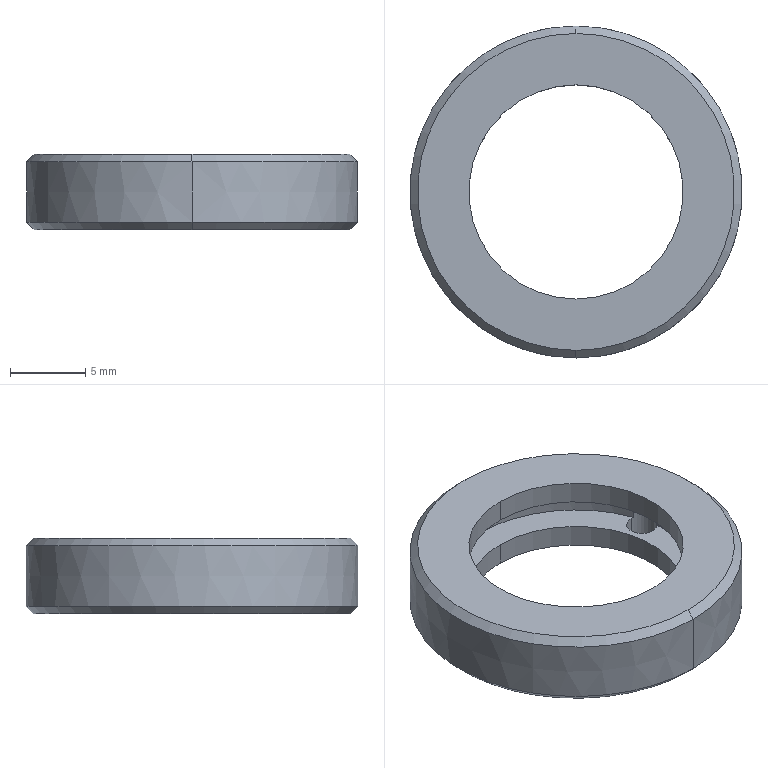Part | SolidWorks | features BaseBody 1 | 1 solid | 22 faces | box 22 x 22 x 5 mm | volume 889.388 mm3 | cylinder 10 | cone 6 | plane 6 | commonest cylinder face diameters 2 x4 14.2 x4 18 x2
STEP:
#1=CARTESIAN_POINT('',(558.371,-163.427,249.045));
#2=VERTEX_POINT('',#1);
#3=CARTESIAN_POINT('',(558.371,-184.426,249.045));
#4=VERTEX_POINT('',#3);
#5=CARTESIAN_POINT('',(558.371,-173.927,249.045));
#6=DIRECTION('',(0.000000003,0.000000023,-1.));
#7=DIRECTION('',(0.,1.,0.000000023));
#8=AXIS2_PLACEMENT_3D('',#5,#6,#7);
#9=CIRCLE('',#8,10.5);
#10=EDGE_CURVE('',#2,#4,#9,.T.);
#11=ORIENTED_EDGE('',*,*,#10,.T.);
#12=CARTESIAN_POINT('',(558.371,-184.926,248.544));
#13=VERTEX_POINT('',#12);
#14=CARTESIAN_POINT('',(558.371,-184.926,248.544));
#15=DIRECTION('',(0.000000002,-0.707,-0.7072));
#16=VECTOR('',#15,1000.);
#17=LINE('',#14,#16);
#18=EDGE_CURVE('',#4,#13,#17,.T.);
#19=ORIENTED_EDGE('',*,*,#18,.T.);
#20=CARTESIAN_POINT('',(558.371,-162.927,248.544));
#21=VERTEX_POINT('',#20);
#22=CARTESIAN_POINT('',(558.371,-173.927,248.544));
#23=DIRECTION('',(-0.000000003,-0.000000023,1.));
#24=DIRECTION('',(-0.9579,-0.287,-0.000000009));
#25=AXIS2_PLACEMENT_3D('',#22,#23,#24);
#26=CIRCLE('',#25,11.);
#27=EDGE_CURVE('',#13,#21,#26,.T.);
#28=ORIENTED_EDGE('',*,*,#27,.T.);
#29=CARTESIAN_POINT('',(558.371,-162.927,248.544));
#30=DIRECTION('',(0.000000002,0.707,-0.7072));
#31=VECTOR('',#30,1000.);
#32=LINE('',#29,#31);
#33=EDGE_CURVE('',#2,#21,#32,.T.);
#34=ORIENTED_EDGE('',*,*,#33,.F.);
#35=EDGE_LOOP('',(#11,#19,#28,#34));
#36=FACE_OUTER_BOUND('',#35,.T.);
#37=CARTESIAN_POINT('',(558.371,-173.927,248.544));
#38=DIRECTION('',(0.000000003,0.000000023,-1.));
#39=DIRECTION('',(0.,1.,0.000000023));
#40=AXIS2_PLACEMENT_3D('',#37,#38,#39);
#41=CONICAL_SURFACE('',#40,11.,0.7853);
#42=ADVANCED_FACE('',(#36),#41,.T.);
#43=CARTESIAN_POINT('',(558.371,-166.827,247.545));
#44=VERTEX_POINT('',#43);
#45=CARTESIAN_POINT('',(558.371,-181.027,247.545));
#46=VERTEX_POINT('',#45);
#47=CARTESIAN_POINT('',(558.371,-173.927,247.545));
#48=DIRECTION('',(-0.000000003,-0.000000023,1.));
#49=DIRECTION('',(0.,-1.,-0.000000023));
#50=AXIS2_PLACEMENT_3D('',#47,#48,#49);
#51=CIRCLE('',#50,7.1);
#52=EDGE_CURVE('',#44,#46,#51,.T.);
#53=ORIENTED_EDGE('',*,*,#52,.F.);
#54=CARTESIAN_POINT('',(558.371,-166.827,249.045));
#55=VERTEX_POINT('',#54);
#56=CARTESIAN_POINT('',(558.371,-166.827,244.045));
#57=DIRECTION('',(-0.000000003,-0.000000023,1.));
#58=VECTOR('',#57,1000.);
#59=LINE('',#56,#58);
#60=EDGE_CURVE('',#44,#55,#59,.T.);
#61=ORIENTED_EDGE('',*,*,#60,.T.);
#62=CARTESIAN_POINT('',(558.371,-181.027,249.045));
#63=VERTEX_POINT('',#62);
#64=CARTESIAN_POINT('',(558.371,-173.927,249.045));
#65=DIRECTION('',(-0.000000003,-0.000000023,1.));
#66=DIRECTION('',(0.,-1.,-0.000000023));
#67=AXIS2_PLACEMENT_3D('',#64,#65,#66);
#68=CIRCLE('',#67,7.1);
#69=EDGE_CURVE('',#55,#63,#68,.T.);
#70=ORIENTED_EDGE('',*,*,#69,.T.);
#71=CARTESIAN_POINT('',(558.371,-181.027,244.045));
#72=DIRECTION('',(-0.000000003,-0.000000023,1.));
#73=VECTOR('',#72,1000.);
#74=LINE('',#71,#73);
#75=EDGE_CURVE('',#46,#63,#74,.T.);
#76=ORIENTED_EDGE('',*,*,#75,.F.);
#77=EDGE_LOOP('',(#53,#61,#70,#76));
#78=FACE_OUTER_BOUND('',#77,.T.);
#79=CARTESIAN_POINT('',(558.371,-173.927,244.045));
#80=DIRECTION('',(-0.000000003,-0.000000023,1.));
#81=DIRECTION('',(0.,-1.,-0.000000023));
#82=AXIS2_PLACEMENT_3D('',#79,#80,#81);
#83=CYLINDRICAL_SURFACE('',#82,7.1);
#84=ADVANCED_FACE('',(#78),#83,.F.);
#85=CARTESIAN_POINT('',(558.371,-184.926,244.545));
#86=VERTEX_POINT('',#85);
#87=CARTESIAN_POINT('',(558.371,-162.927,244.545));
#88=VERTEX_POINT('',#87);
#89=CARTESIAN_POINT('',(558.371,-173.927,244.545));
#90=DIRECTION('',(-0.000000003,-0.000000023,1.));
#91=DIRECTION('',(-0.9579,-0.287,-0.000000009));
#92=AXIS2_PLACEMENT_3D('',#89,#90,#91);
#93=CIRCLE('',#92,10.999);
#94=EDGE_CURVE('',#86,#88,#93,.T.);
#95=ORIENTED_EDGE('',*,*,#94,.T.);
#96=CARTESIAN_POINT('',(558.371,-162.927,248.544));
#97=DIRECTION('',(-0.000000003,0.0001745,1.));
#98=VECTOR('',#97,1000.);
#99=LINE('',#96,#98);
#100=EDGE_CURVE('',#88,#21,#99,.T.);
#101=ORIENTED_EDGE('',*,*,#100,.T.);
#102=ORIENTED_EDGE('',*,*,#27,.F.);
#103=CARTESIAN_POINT('',(558.371,-184.926,248.544));
#104=DIRECTION('',(-0.000000003,-0.0001746,1.));
#105=VECTOR('',#104,1000.);
#106=LINE('',#103,#105);
#107=EDGE_CURVE('',#86,#13,#106,.T.);
#108=ORIENTED_EDGE('',*,*,#107,.F.);
#109=EDGE_LOOP('',(#95,#101,#102,#108));
#110=FACE_OUTER_BOUND('',#109,.T.);
#111=CARTESIAN_POINT('',(558.371,-173.927,248.544));
#112=DIRECTION('',(-0.000000003,-0.000000023,1.));
#113=DIRECTION('',(0.,-1.,-0.000000023));
#114=AXIS2_PLACEMENT_3D('',#111,#112,#113);
#115=CONICAL_SURFACE('',#114,11.,0.0001745);
#116=ADVANCED_FACE('',(#110),#115,.T.);
#117=CARTESIAN_POINT('',(558.371,-184.426,244.045));
#118=VERTEX_POINT('',#117);
#119=CARTESIAN_POINT('',(558.371,-163.427,244.045));
#120=VERTEX_POINT('',#119);
#121=CARTESIAN_POINT('',(558.371,-173.927,244.045));
#122=DIRECTION('',(-0.000000003,-0.000000023,1.));
#123=DIRECTION('',(0.,-1.,-0.000000023));
#124=AXIS2_PLACEMENT_3D('',#121,#122,#123);
#125=CIRCLE('',#124,10.499);
#126=EDGE_CURVE('',#118,#120,#125,.T.);
#127=ORIENTED_EDGE('',*,*,#126,.T.);
#128=CARTESIAN_POINT('',(558.371,-162.927,244.545));
#129=DIRECTION('',(-0.000000002,0.7072,0.707));
#130=VECTOR('',#129,1000.);
#131=LINE('',#128,#130);
#132=EDGE_CURVE('',#120,#88,#131,.T.);
#133=ORIENTED_EDGE('',*,*,#132,.T.);
#134=ORIENTED_EDGE('',*,*,#94,.F.);
#135=CARTESIAN_POINT('',(558.371,-184.926,244.545));
#136=DIRECTION('',(-0.000000002,-0.7072,0.707));
#137=VECTOR('',#136,1000.);
#138=LINE('',#135,#137);
#139=EDGE_CURVE('',#118,#86,#138,.T.);
#140=ORIENTED_EDGE('',*,*,#139,.F.);
#141=EDGE_LOOP('',(#127,#133,#134,#140));
#142=FACE_OUTER_BOUND('',#141,.T.);
#143=CARTESIAN_POINT('',(558.371,-173.927,244.545));
#144=DIRECTION('',(-0.000000003,-0.000000023,1.));
#145=DIRECTION('',(0.,-1.,-0.000000023));
#146=AXIS2_PLACEMENT_3D('',#143,#144,#145);
#147=CONICAL_SURFACE('',#146,10.999,0.7855);
#148=ADVANCED_FACE('',(#142),#147,.T.);
#149=CARTESIAN_POINT('',(558.371,-164.927,247.545));
#150=VERTEX_POINT('',#149);
#151=CARTESIAN_POINT('',(558.371,-182.927,247.545));
#152=VERTEX_POINT('',#151);
#153=CARTESIAN_POINT('',(558.371,-173.927,247.545));
#154=DIRECTION('',(-0.000000003,-0.000000023,1.));
#155=DIRECTION('',(0.,1.,0.000000023));
#156=AXIS2_PLACEMENT_3D('',#153,#154,#155);
#157=CIRCLE('',#156,9.);
#158=EDGE_CURVE('',#150,#152,#157,.T.);
#159=ORIENTED_EDGE('',*,*,#158,.T.);
#160=CARTESIAN_POINT('',(558.371,-182.927,245.545));
#161=VERTEX_POINT('',#160);
#162=CARTESIAN_POINT('',(558.371,-182.927,245.545));
#163=DIRECTION('',(0.000000003,0.000000023,-1.));
#164=VECTOR('',#163,1000.);
#165=LINE('',#162,#164);
#166=EDGE_CURVE('',#152,#161,#165,.T.);
#167=ORIENTED_EDGE('',*,*,#166,.T.);
#168=CARTESIAN_POINT('',(549.904,-176.978,245.545));
#169=VERTEX_POINT('',#168);
#170=CARTESIAN_POINT('',(558.371,-173.927,245.545));
#171=DIRECTION('',(-0.000000003,-0.000000023,1.));
#172=DIRECTION('',(0.,1.,0.000000023));
#173=AXIS2_PLACEMENT_3D('',#170,#171,#172);
#174=CIRCLE('',#173,9.);
#175=EDGE_CURVE('',#169,#161,#174,.T.);
#176=ORIENTED_EDGE('',*,*,#175,.F.);
#177=CARTESIAN_POINT('',(549.904,-176.978,246.045));
#178=VERTEX_POINT('',#177);
#179=CARTESIAN_POINT('',(549.904,-176.978,244.045));
#180=DIRECTION('',(-0.000000003,-0.000000023,1.));
#181=VECTOR('',#180,1000.);
#182=LINE('',#179,#181);
#183=EDGE_CURVE('',#169,#178,#182,.T.);
#184=ORIENTED_EDGE('',*,*,#183,.T.);
#185=CARTESIAN_POINT('',(549.469,-175.252,246.045));
#186=VERTEX_POINT('',#185);
#187=CARTESIAN_POINT('',(558.371,-173.927,246.045));
#188=DIRECTION('',(-0.000000003,-0.000000023,1.));
#189=DIRECTION('',(0.,1.,0.000000023));
#190=AXIS2_PLACEMENT_3D('',#187,#188,#189);
#191=CIRCLE('',#190,9.);
#192=EDGE_CURVE('',#186,#178,#191,.T.);
#193=ORIENTED_EDGE('',*,*,#192,.F.);
#194=CARTESIAN_POINT('',(549.469,-175.252,245.545));
#195=VERTEX_POINT('',#194);
#196=CARTESIAN_POINT('',(549.469,-175.252,244.045));
#197=DIRECTION('',(0.000000003,0.000000023,-1.));
#198=VECTOR('',#197,1000.);
#199=LINE('',#196,#198);
#200=EDGE_CURVE('',#186,#195,#199,.T.);
#201=ORIENTED_EDGE('',*,*,#200,.T.);
#202=CARTESIAN_POINT('',(558.371,-164.927,245.545));
#203=VERTEX_POINT('',#202);
#204=CARTESIAN_POINT('',(558.371,-173.927,245.545));
#205=DIRECTION('',(-0.000000003,-0.000000023,1.));
#206=DIRECTION('',(0.,1.,0.000000023));
#207=AXIS2_PLACEMENT_3D('',#204,#205,#206);
#208=CIRCLE('',#207,9.);
#209=EDGE_CURVE('',#203,#195,#208,.T.);
#210=ORIENTED_EDGE('',*,*,#209,.F.);
#211=CARTESIAN_POINT('',(558.371,-164.927,245.545));
#212=DIRECTION('',(0.000000003,0.000000023,-1.));
#213=VECTOR('',#212,1000.);
#214=LINE('',#211,#213);
#215=EDGE_CURVE('',#150,#203,#214,.T.);
#216=ORIENTED_EDGE('',*,*,#215,.F.);
#217=EDGE_LOOP('',(#159,#167,#176,#184,#193,#201,#210,#216));
#218=FACE_OUTER_BOUND('',#217,.T.);
#219=CARTESIAN_POINT('',(558.371,-173.927,245.545));
#220=DIRECTION('',(0.000000003,0.000000023,-1.));
#221=DIRECTION('',(0.,1.,0.000000023));
#222=AXIS2_PLACEMENT_3D('',#219,#220,#221);
#223=CYLINDRICAL_SURFACE('',#222,9.);
#224=ADVANCED_FACE('',(#218),#223,.F.);
#225=CARTESIAN_POINT('',(558.371,-166.827,244.045));
#226=VERTEX_POINT('',#225);
#227=CARTESIAN_POINT('',(558.371,-181.027,244.045));
#228=VERTEX_POINT('',#227);
#229=CARTESIAN_POINT('',(558.371,-173.927,244.045));
#230=DIRECTION('',(-0.000000003,-0.000000023,1.));
#231=DIRECTION('',(0.,-1.,-0.000000023));
#232=AXIS2_PLACEMENT_3D('',#229,#230,#231);
#233=CIRCLE('',#232,7.1);
#234=EDGE_CURVE('',#226,#228,#233,.T.);
#235=ORIENTED_EDGE('',*,*,#234,.F.);
#236=CARTESIAN_POINT('',(558.371,-166.827,245.545));
#237=VERTEX_POINT('',#236);
#238=CARTESIAN_POINT('',(558.371,-166.827,244.045));
#239=DIRECTION('',(-0.000000003,-0.000000023,1.));
#240=VECTOR('',#239,1000.);
#241=LINE('',#238,#240);
#242=EDGE_CURVE('',#226,#237,#241,.T.);
#243=ORIENTED_EDGE('',*,*,#242,.T.);
#244=CARTESIAN_POINT('',(558.371,-181.027,245.545));
#245=VERTEX_POINT('',#244);
#246=CARTESIAN_POINT('',(558.371,-173.927,245.545));
#247=DIRECTION('',(0.000000003,0.000000023,-1.));
#248=DIRECTION('',(0.,-1.,-0.000000023));
#249=AXIS2_PLACEMENT_3D('',#246,#247,#248);
#250=CIRCLE('',#249,7.1);
#251=EDGE_CURVE('',#245,#237,#250,.T.);
#252=ORIENTED_EDGE('',*,*,#251,.F.);
#253=CARTESIAN_POINT('',(558.371,-181.027,244.045));
#254=DIRECTION('',(-0.000000003,-0.000000023,1.));
#255=VECTOR('',#254,1000.);
#256=LINE('',#253,#255);
#257=EDGE_CURVE('',#228,#245,#256,.T.);
#258=ORIENTED_EDGE('',*,*,#257,.F.);
#259=EDGE_LOOP('',(#235,#243,#252,#258));
#260=FACE_OUTER_BOUND('',#259,.T.);
#261=CARTESIAN_POINT('',(558.371,-173.927,244.045));
#262=DIRECTION('',(-0.000000003,-0.000000023,1.));
#263=DIRECTION('',(0.,-1.,-0.000000023));
#264=AXIS2_PLACEMENT_3D('',#261,#262,#263);
#265=CYLINDRICAL_SURFACE('',#264,7.1);
#266=ADVANCED_FACE('',(#260),#265,.F.);
#267=CARTESIAN_POINT('',(566.613,-172.849,245.545));
#268=VERTEX_POINT('',#267);
#269=CARTESIAN_POINT('',(566.613,-170.849,245.545));
#270=VERTEX_POINT('',#269);
#271=CARTESIAN_POINT('',(566.613,-171.849,245.545));
#272=DIRECTION('',(0.000000003,0.000000023,-1.));
#273=DIRECTION('',(0.,1.,0.000000023));
#274=AXIS2_PLACEMENT_3D('',#271,#272,#273);
#275=CIRCLE('',#274,1.);
#276=EDGE_CURVE('',#268,#270,#275,.T.);
#277=ORIENTED_EDGE('',*,*,#276,.F.);
#278=CARTESIAN_POINT('',(566.613,-172.849,244.045));
#279=VERTEX_POINT('',#278);
#280=CARTESIAN_POINT('',(566.613,-172.849,244.045));
#281=DIRECTION('',(0.000000003,0.000000023,-1.));
#282=VECTOR('',#281,1000.);
#283=LINE('',#280,#282);
#284=EDGE_CURVE('',#268,#279,#283,.T.);
#285=ORIENTED_EDGE('',*,*,#284,.T.);
#286=CARTESIAN_POINT('',(566.613,-170.849,244.045));
#287=VERTEX_POINT('',#286);
#288=CARTESIAN_POINT('',(566.613,-171.849,244.045));
#289=DIRECTION('',(-0.000000003,-0.000000023,1.));
#290=DIRECTION('',(0.,1.,0.000000023));
#291=AXIS2_PLACEMENT_3D('',#288,#289,#290);
#292=CIRCLE('',#291,1.);
#293=EDGE_CURVE('',#287,#279,#292,.T.);
#294=ORIENTED_EDGE('',*,*,#293,.F.);
#295=CARTESIAN_POINT('',(566.613,-170.849,244.045));
#296=DIRECTION('',(0.000000003,0.000000023,-1.));
#297=VECTOR('',#296,1000.);
#298=LINE('',#295,#297);
#299=EDGE_CURVE('',#270,#287,#298,.T.);
#300=ORIENTED_EDGE('',*,*,#299,.F.);
#301=EDGE_LOOP('',(#277,#285,#294,#300));
#302=FACE_OUTER_BOUND('',#301,.T.);
#303=CARTESIAN_POINT('',(566.613,-171.849,244.045));
#304=DIRECTION('',(0.000000003,0.000000023,-1.));
#305=DIRECTION('',(0.,1.,0.000000023));
#306=AXIS2_PLACEMENT_3D('',#303,#304,#305);
#307=CYLINDRICAL_SURFACE('',#306,1.);
#308=ADVANCED_FACE('',(#302),#307,.F.);
#309=CARTESIAN_POINT('',(550.129,-177.004,245.545));
#310=VERTEX_POINT('',#309);
#311=CARTESIAN_POINT('',(550.129,-176.004,245.545));
#312=DIRECTION('',(0.000000003,0.000000023,-1.));
#313=DIRECTION('',(0.,1.,0.000000023));
#314=AXIS2_PLACEMENT_3D('',#311,#312,#313);
#315=CIRCLE('',#314,1.);
#316=EDGE_CURVE('',#310,#169,#315,.T.);
#317=ORIENTED_EDGE('',*,*,#316,.F.);
#318=CARTESIAN_POINT('',(550.129,-177.004,244.045));
#319=VERTEX_POINT('',#318);
#320=CARTESIAN_POINT('',(550.129,-177.004,244.045));
#321=DIRECTION('',(0.000000003,0.000000023,-1.));
#322=VECTOR('',#321,1000.);
#323=LINE('',#320,#322);
#324=EDGE_CURVE('',#310,#319,#323,.T.);
#325=ORIENTED_EDGE('',*,*,#324,.T.);
#326=CARTESIAN_POINT('',(550.129,-175.004,244.045));
#327=VERTEX_POINT('',#326);
#328=CARTESIAN_POINT('',(550.129,-176.004,244.045));
#329=DIRECTION('',(-0.000000003,-0.000000023,1.));
#330=DIRECTION('',(0.,1.,0.000000023));
#331=AXIS2_PLACEMENT_3D('',#328,#329,#330);
#332=CIRCLE('',#331,1.);
#333=EDGE_CURVE('',#327,#319,#332,.T.);
#334=ORIENTED_EDGE('',*,*,#333,.F.);
#335=CARTESIAN_POINT('',(550.129,-175.004,245.545));
#336=VERTEX_POINT('',#335);
#337=CARTESIAN_POINT('',(550.129,-175.004,244.045));
#338=DIRECTION('',(0.000000003,0.000000023,-1.));
#339=VECTOR('',#338,1000.);
#340=LINE('',#337,#339);
#341=EDGE_CURVE('',#336,#327,#340,.T.);
#342=ORIENTED_EDGE('',*,*,#341,.F.);
#343=CARTESIAN_POINT('',(550.129,-176.004,245.545));
#344=DIRECTION('',(0.000000003,0.000000023,-1.));
#345=DIRECTION('',(0.,1.,0.000000023));
#346=AXIS2_PLACEMENT_3D('',#343,#344,#345);
#347=CIRCLE('',#346,1.);
#348=EDGE_CURVE('',#195,#336,#347,.T.);
#349=ORIENTED_EDGE('',*,*,#348,.F.);
#350=ORIENTED_EDGE('',*,*,#200,.F.);
#351=CARTESIAN_POINT('',(550.129,-176.004,246.045));
#352=DIRECTION('',(-0.000000003,-0.000000023,1.));
#353=DIRECTION('',(0.,1.,0.000000023));
#354=AXIS2_PLACEMENT_3D('',#351,#352,#353);
#355=CIRCLE('',#354,1.);
#356=EDGE_CURVE('',#186,#178,#355,.T.);
#357=ORIENTED_EDGE('',*,*,#356,.T.);
#358=ORIENTED_EDGE('',*,*,#183,.F.);
#359=EDGE_LOOP('',(#317,#325,#334,#342,#349,#350,#357,#358));
#360=FACE_OUTER_BOUND('',#359,.T.);
#361=CARTESIAN_POINT('',(550.129,-176.004,244.045));
#362=DIRECTION('',(0.000000003,0.000000023,-1.));
#363=DIRECTION('',(0.,1.,0.000000023));
#364=AXIS2_PLACEMENT_3D('',#361,#362,#363);
#365=CYLINDRICAL_SURFACE('',#364,1.);
#366=ADVANCED_FACE('',(#360),#365,.F.);
#367=ORIENTED_EDGE('',*,*,#10,.F.);
#368=CARTESIAN_POINT('',(558.371,-173.927,249.045));
#369=DIRECTION('',(0.000000003,0.000000023,-1.));
#370=DIRECTION('',(0.,1.,0.000000023));
#371=AXIS2_PLACEMENT_3D('',#368,#369,#370);
#372=CIRCLE('',#371,10.5);
#373=EDGE_CURVE('',#4,#2,#372,.T.);
#374=ORIENTED_EDGE('',*,*,#373,.F.);
#375=EDGE_LOOP('',(#367,#374));
#376=FACE_OUTER_BOUND('',#375,.T.);
#377=CARTESIAN_POINT('',(558.371,-173.927,249.045));
#378=DIRECTION('',(-0.000000003,-0.000000023,1.));
#379=DIRECTION('',(0.,-1.,-0.000000023));
#380=AXIS2_PLACEMENT_3D('',#377,#378,#379);
#381=CIRCLE('',#380,7.1);
#382=EDGE_CURVE('',#63,#55,#381,.T.);
#383=ORIENTED_EDGE('',*,*,#382,.F.);
#384=ORIENTED_EDGE('',*,*,#69,.F.);
#385=EDGE_LOOP('',(#383,#384));
#386=FACE_BOUND('',#385,.T.);
#387=CARTESIAN_POINT('',(558.371,-173.927,249.045));
#388=DIRECTION('',(0.000000003,0.000000023,-1.));
#389=DIRECTION('',(0.,1.,0.000000023));
#390=AXIS2_PLACEMENT_3D('',#387,#388,#389);
#391=PLANE('',#390);
#392=ADVANCED_FACE('',(#376,#386),#391,.F.);
#393=ORIENTED_EDGE('',*,*,#18,.F.);
#394=ORIENTED_EDGE('',*,*,#373,.T.);
#395=ORIENTED_EDGE('',*,*,#33,.T.);
#396=CARTESIAN_POINT('',(558.371,-173.927,248.544));
#397=DIRECTION('',(-0.000000003,-0.000000023,1.));
#398=DIRECTION('',(-0.9579,-0.287,-0.000000009));
#399=AXIS2_PLACEMENT_3D('',#396,#397,#398);
#400=CIRCLE('',#399,11.);
#401=EDGE_CURVE('',#21,#13,#400,.T.);
#402=ORIENTED_EDGE('',*,*,#401,.T.);
#403=EDGE_LOOP('',(#393,#394,#395,#402));
#404=FACE_OUTER_BOUND('',#403,.T.);
#405=CARTESIAN_POINT('',(558.371,-173.927,248.544));
#406=DIRECTION('',(0.000000003,0.000000023,-1.));
#407=DIRECTION('',(0.,1.,0.000000023));
#408=AXIS2_PLACEMENT_3D('',#405,#406,#407);
#409=CONICAL_SURFACE('',#408,11.,0.7853);
#410=ADVANCED_FACE('',(#404),#409,.T.);
#411=ORIENTED_EDGE('',*,*,#60,.F.);
#412=CARTESIAN_POINT('',(558.371,-173.927,247.545));
#413=DIRECTION('',(-0.000000003,-0.000000023,1.));
#414=DIRECTION('',(0.,-1.,-0.000000023));
#415=AXIS2_PLACEMENT_3D('',#412,#413,#414);
#416=CIRCLE('',#415,7.1);
#417=EDGE_CURVE('',#46,#44,#416,.T.);
#418=ORIENTED_EDGE('',*,*,#417,.F.);
#419=ORIENTED_EDGE('',*,*,#75,.T.);
#420=ORIENTED_EDGE('',*,*,#382,.T.);
#421=EDGE_LOOP('',(#411,#418,#419,#420));
#422=FACE_OUTER_BOUND('',#421,.T.);
#423=CARTESIAN_POINT('',(558.371,-173.927,244.045));
#424=DIRECTION('',(-0.000000003,-0.000000023,1.));
#425=DIRECTION('',(0.,-1.,-0.000000023));
#426=AXIS2_PLACEMENT_3D('',#423,#424,#425);
#427=CYLINDRICAL_SURFACE('',#426,7.1);
#428=ADVANCED_FACE('',(#422),#427,.F.);
#429=ORIENTED_EDGE('',*,*,#100,.F.);
#430=CARTESIAN_POINT('',(558.371,-173.927,244.545));
#431=DIRECTION('',(-0.000000003,-0.000000023,1.));
#432=DIRECTION('',(-0.9579,-0.287,-0.000000009));
#433=AXIS2_PLACEMENT_3D('',#430,#431,#432);
#434=CIRCLE('',#433,10.999);
#435=EDGE_CURVE('',#88,#86,#434,.T.);
#436=ORIENTED_EDGE('',*,*,#435,.T.);
#437=ORIENTED_EDGE('',*,*,#107,.T.);
#438=ORIENTED_EDGE('',*,*,#401,.F.);
#439=EDGE_LOOP('',(#429,#436,#437,#438));
#440=FACE_OUTER_BOUND('',#439,.T.);
#441=CARTESIAN_POINT('',(558.371,-173.927,248.544));
#442=DIRECTION('',(-0.000000003,-0.000000023,1.));
#443=DIRECTION('',(0.,-1.,-0.000000023));
#444=AXIS2_PLACEMENT_3D('',#441,#442,#443);
#445=CONICAL_SURFACE('',#444,11.,0.0001745);
#446=ADVANCED_FACE('',(#440),#445,.T.);
#447=ORIENTED_EDGE('',*,*,#158,.F.);
#448=CARTESIAN_POINT('',(558.371,-173.927,247.545));
#449=DIRECTION('',(-0.000000003,-0.000000023,1.));
#450=DIRECTION('',(0.,1.,0.000000023));
#451=AXIS2_PLACEMENT_3D('',#448,#449,#450);
#452=CIRCLE('',#451,9.);
#453=EDGE_CURVE('',#152,#150,#452,.T.);
#454=ORIENTED_EDGE('',*,*,#453,.F.);
#455=EDGE_LOOP('',(#447,#454));
#456=FACE_OUTER_BOUND('',#455,.T.);
#457=ORIENTED_EDGE('',*,*,#417,.T.);
#458=ORIENTED_EDGE('',*,*,#52,.T.);
#459=EDGE_LOOP('',(#457,#458));
#460=FACE_BOUND('',#459,.T.);
#461=CARTESIAN_POINT('',(558.371,-173.927,247.545));
#462=DIRECTION('',(-0.000000003,-0.000000023,1.));
#463=DIRECTION('',(0.,-1.,-0.000000023));
#464=AXIS2_PLACEMENT_3D('',#461,#462,#463);
#465=PLANE('',#464);
#466=ADVANCED_FACE('',(#456,#460),#465,.F.);
#467=ORIENTED_EDGE('',*,*,#132,.F.);
#468=CARTESIAN_POINT('',(558.371,-173.927,244.045));
#469=DIRECTION('',(-0.000000003,-0.000000023,1.));
#470=DIRECTION('',(0.,-1.,-0.000000023));
#471=AXIS2_PLACEMENT_3D('',#468,#469,#470);
#472=CIRCLE('',#471,10.499);
#473=EDGE_CURVE('',#120,#118,#472,.T.);
#474=ORIENTED_EDGE('',*,*,#473,.T.);
#475=ORIENTED_EDGE('',*,*,#139,.T.);
#476=ORIENTED_EDGE('',*,*,#435,.F.);
#477=EDGE_LOOP('',(#467,#474,#475,#476));
#478=FACE_OUTER_BOUND('',#477,.T.);
#479=CARTESIAN_POINT('',(558.371,-173.927,244.545));
#480=DIRECTION('',(-0.000000003,-0.000000023,1.));
#481=DIRECTION('',(0.,-1.,-0.000000023));
#482=AXIS2_PLACEMENT_3D('',#479,#480,#481);
#483=CONICAL_SURFACE('',#482,10.999,0.7855);
#484=ADVANCED_FACE('',(#478),#483,.T.);
#485=ORIENTED_EDGE('',*,*,#166,.F.);
#486=ORIENTED_EDGE('',*,*,#453,.T.);
#487=ORIENTED_EDGE('',*,*,#215,.T.);
#488=CARTESIAN_POINT('',(566.838,-170.875,245.545));
#489=VERTEX_POINT('',#488);
#490=CARTESIAN_POINT('',(558.371,-173.927,245.545));
#491=DIRECTION('',(-0.000000003,-0.000000023,1.));
#492=DIRECTION('',(0.,1.,0.000000023));
#493=AXIS2_PLACEMENT_3D('',#490,#491,#492);
#494=CIRCLE('',#493,9.);
#495=EDGE_CURVE('',#489,#203,#494,.T.);
#496=ORIENTED_EDGE('',*,*,#495,.F.);
#497=CARTESIAN_POINT('',(566.838,-170.875,246.045));
#498=VERTEX_POINT('',#497);
#499=CARTESIAN_POINT('',(566.838,-170.875,244.045));
#500=DIRECTION('',(-0.000000003,-0.000000023,1.));
#501=VECTOR('',#500,1000.);
#502=LINE('',#499,#501);
#503=EDGE_CURVE('',#489,#498,#502,.T.);
#504=ORIENTED_EDGE('',*,*,#503,.T.);
#505=CARTESIAN_POINT('',(567.273,-172.601,246.045));
#506=VERTEX_POINT('',#505);
#507=CARTESIAN_POINT('',(558.371,-173.927,246.045));
#508=DIRECTION('',(-0.000000003,-0.000000023,1.));
#509=DIRECTION('',(0.,1.,0.000000023));
#510=AXIS2_PLACEMENT_3D('',#507,#508,#509);
#511=CIRCLE('',#510,9.);
#512=EDGE_CURVE('',#506,#498,#511,.T.);
#513=ORIENTED_EDGE('',*,*,#512,.F.);
#514=CARTESIAN_POINT('',(567.273,-172.601,245.545));
#515=VERTEX_POINT('',#514);
#516=CARTESIAN_POINT('',(567.273,-172.601,244.045));
#517=DIRECTION('',(0.000000003,0.000000023,-1.));
#518=VECTOR('',#517,1000.);
#519=LINE('',#516,#518);
#520=EDGE_CURVE('',#506,#515,#519,.T.);
#521=ORIENTED_EDGE('',*,*,#520,.T.);
#522=CARTESIAN_POINT('',(558.371,-173.927,245.545));
#523=DIRECTION('',(-0.000000003,-0.000000023,1.));
#524=DIRECTION('',(0.,1.,0.000000023));
#525=AXIS2_PLACEMENT_3D('',#522,#523,#524);
#526=CIRCLE('',#525,9.);
#527=EDGE_CURVE('',#161,#515,#526,.T.);
#528=ORIENTED_EDGE('',*,*,#527,.F.);
#529=EDGE_LOOP('',(#485,#486,#487,#496,#504,#513,#521,#528));
#530=FACE_OUTER_BOUND('',#529,.T.);
#531=CARTESIAN_POINT('',(558.371,-173.927,245.545));
#532=DIRECTION('',(0.000000003,0.000000023,-1.));
#533=DIRECTION('',(0.,1.,0.000000023));
#534=AXIS2_PLACEMENT_3D('',#531,#532,#533);
#535=CYLINDRICAL_SURFACE('',#534,9.);
#536=ADVANCED_FACE('',(#530),#535,.F.);
#537=ORIENTED_EDGE('',*,*,#126,.F.);
#538=ORIENTED_EDGE('',*,*,#473,.F.);
#539=EDGE_LOOP('',(#537,#538));
#540=FACE_OUTER_BOUND('',#539,.T.);
#541=CARTESIAN_POINT('',(558.371,-173.927,244.045));
#542=DIRECTION('',(-0.000000003,-0.000000023,1.));
#543=DIRECTION('',(0.,-1.,-0.000000023));
#544=AXIS2_PLACEMENT_3D('',#541,#542,#543);
#545=CIRCLE('',#544,7.1);
#546=EDGE_CURVE('',#228,#226,#545,.T.);
#547=ORIENTED_EDGE('',*,*,#546,.T.);
#548=ORIENTED_EDGE('',*,*,#234,.T.);
#549=EDGE_LOOP('',(#547,#548));
#550=FACE_BOUND('',#549,.T.);
#551=ORIENTED_EDGE('',*,*,#293,.T.);
#552=CARTESIAN_POINT('',(566.613,-171.849,244.045));
#553=DIRECTION('',(-0.000000003,-0.000000023,1.));
#554=DIRECTION('',(0.,1.,0.000000023));
#555=AXIS2_PLACEMENT_3D('',#552,#553,#554);
#556=CIRCLE('',#555,1.);
#557=EDGE_CURVE('',#279,#287,#556,.T.);
#558=ORIENTED_EDGE('',*,*,#557,.T.);
#559=EDGE_LOOP('',(#551,#558));
#560=FACE_BOUND('',#559,.T.);
#561=ORIENTED_EDGE('',*,*,#333,.T.);
#562=CARTESIAN_POINT('',(550.129,-176.004,244.045));
#563=DIRECTION('',(-0.000000003,-0.000000023,1.));
#564=DIRECTION('',(0.,1.,0.000000023));
#565=AXIS2_PLACEMENT_3D('',#562,#563,#564);
#566=CIRCLE('',#565,1.);
#567=EDGE_CURVE('',#319,#327,#566,.T.);
#568=ORIENTED_EDGE('',*,*,#567,.T.);
#569=EDGE_LOOP('',(#561,#568));
#570=FACE_BOUND('',#569,.T.);
#571=CARTESIAN_POINT('',(558.371,-173.927,244.045));
#572=DIRECTION('',(0.000000003,0.000000023,-1.));
#573=DIRECTION('',(0.,1.,0.000000023));
#574=AXIS2_PLACEMENT_3D('',#571,#572,#573);
#575=PLANE('',#574);
#576=ADVANCED_FACE('',(#540,#550,#560,#570),#575,.T.);
#577=ORIENTED_EDGE('',*,*,#356,.F.);
#578=ORIENTED_EDGE('',*,*,#192,.T.);
#579=EDGE_LOOP('',(#577,#578));
#580=FACE_OUTER_BOUND('',#579,.T.);
#581=CARTESIAN_POINT('',(550.129,-176.004,246.045));
#582=DIRECTION('',(-0.000000003,-0.000000023,1.));
#583=DIRECTION('',(0.,-1.,-0.000000023));
#584=AXIS2_PLACEMENT_3D('',#581,#582,#583);
#585=PLANE('',#584);
#586=ADVANCED_FACE('',(#580),#585,.F.);
#587=ORIENTED_EDGE('',*,*,#251,.T.);
#588=CARTESIAN_POINT('',(558.371,-173.927,245.545));
#589=DIRECTION('',(0.000000003,0.000000023,-1.));
#590=DIRECTION('',(0.,-1.,-0.000000023));
#591=AXIS2_PLACEMENT_3D('',#588,#589,#590);
#592=CIRCLE('',#591,7.1);
#593=EDGE_CURVE('',#237,#245,#592,.T.);
#594=ORIENTED_EDGE('',*,*,#593,.T.);
#595=EDGE_LOOP('',(#587,#594));
#596=FACE_BOUND('',#595,.T.);
#597=CARTESIAN_POINT('',(566.613,-171.849,245.545));
#598=DIRECTION('',(0.000000003,0.000000023,-1.));
#599=DIRECTION('',(0.,1.,0.000000023));
#600=AXIS2_PLACEMENT_3D('',#597,#598,#599);
#601=CIRCLE('',#600,1.);
#602=EDGE_CURVE('',#515,#268,#601,.T.);
#603=ORIENTED_EDGE('',*,*,#602,.T.);
#604=ORIENTED_EDGE('',*,*,#276,.T.);
#605=CARTESIAN_POINT('',(566.613,-171.849,245.545));
#606=DIRECTION('',(0.000000003,0.000000023,-1.));
#607=DIRECTION('',(0.,1.,0.000000023));
#608=AXIS2_PLACEMENT_3D('',#605,#606,#607);
#609=CIRCLE('',#608,1.);
#610=EDGE_CURVE('',#270,#489,#609,.T.);
#611=ORIENTED_EDGE('',*,*,#610,.T.);
#612=ORIENTED_EDGE('',*,*,#495,.T.);
#613=ORIENTED_EDGE('',*,*,#209,.T.);
#614=ORIENTED_EDGE('',*,*,#348,.T.);
#615=CARTESIAN_POINT('',(550.129,-176.004,245.545));
#616=DIRECTION('',(0.000000003,0.000000023,-1.));
#617=DIRECTION('',(0.,1.,0.000000023));
#618=AXIS2_PLACEMENT_3D('',#615,#616,#617);
#619=CIRCLE('',#618,1.);
#620=EDGE_CURVE('',#336,#310,#619,.T.);
#621=ORIENTED_EDGE('',*,*,#620,.T.);
#622=ORIENTED_EDGE('',*,*,#316,.T.);
#623=ORIENTED_EDGE('',*,*,#175,.T.);
#624=ORIENTED_EDGE('',*,*,#527,.T.);
#625=EDGE_LOOP('',(#603,#604,#611,#612,#613,#614,#621,#622,#623,#624));
#626=FACE_OUTER_BOUND('',#625,.T.);
#627=CARTESIAN_POINT('',(558.371,-173.927,245.545));
#628=DIRECTION('',(-0.000000003,-0.000000023,1.));
#629=DIRECTION('',(0.,-1.,-0.000000023));
#630=AXIS2_PLACEMENT_3D('',#627,#628,#629);
#631=PLANE('',#630);
#632=ADVANCED_FACE('',(#596,#626),#631,.T.);
#633=CARTESIAN_POINT('',(566.613,-171.849,246.045));
#634=DIRECTION('',(-0.000000003,-0.000000023,1.));
#635=DIRECTION('',(0.,1.,0.000000023));
#636=AXIS2_PLACEMENT_3D('',#633,#634,#635);
#637=CIRCLE('',#636,1.);
#638=EDGE_CURVE('',#506,#498,#637,.T.);
#639=ORIENTED_EDGE('',*,*,#638,.F.);
#640=ORIENTED_EDGE('',*,*,#512,.T.);
#641=EDGE_LOOP('',(#639,#640));
#642=FACE_OUTER_BOUND('',#641,.T.);
#643=CARTESIAN_POINT('',(566.613,-171.849,246.045));
#644=DIRECTION('',(-0.000000003,-0.000000023,1.));
#645=DIRECTION('',(0.,-1.,-0.000000023));
#646=AXIS2_PLACEMENT_3D('',#643,#644,#645);
#647=PLANE('',#646);
#648=ADVANCED_FACE('',(#642),#647,.F.);
#649=ORIENTED_EDGE('',*,*,#242,.F.);
#650=ORIENTED_EDGE('',*,*,#546,.F.);
#651=ORIENTED_EDGE('',*,*,#257,.T.);
#652=ORIENTED_EDGE('',*,*,#593,.F.);
#653=EDGE_LOOP('',(#649,#650,#651,#652));
#654=FACE_OUTER_BOUND('',#653,.T.);
#655=CARTESIAN_POINT('',(558.371,-173.927,244.045));
#656=DIRECTION('',(-0.000000003,-0.000000023,1.));
#657=DIRECTION('',(0.,-1.,-0.000000023));
#658=AXIS2_PLACEMENT_3D('',#655,#656,#657);
#659=CYLINDRICAL_SURFACE('',#658,7.1);
#660=ADVANCED_FACE('',(#654),#659,.F.);
#661=ORIENTED_EDGE('',*,*,#284,.F.);
#662=ORIENTED_EDGE('',*,*,#602,.F.);
#663=ORIENTED_EDGE('',*,*,#520,.F.);
#664=ORIENTED_EDGE('',*,*,#638,.T.);
#665=ORIENTED_EDGE('',*,*,#503,.F.);
#666=ORIENTED_EDGE('',*,*,#610,.F.);
#667=ORIENTED_EDGE('',*,*,#299,.T.);
#668=ORIENTED_EDGE('',*,*,#557,.F.);
#669=EDGE_LOOP('',(#661,#662,#663,#664,#665,#666,#667,#668));
#670=FACE_OUTER_BOUND('',#669,.T.);
#671=CARTESIAN_POINT('',(566.613,-171.849,244.045));
#672=DIRECTION('',(0.000000003,0.000000023,-1.));
#673=DIRECTION('',(0.,1.,0.000000023));
#674=AXIS2_PLACEMENT_3D('',#671,#672,#673);
#675=CYLINDRICAL_SURFACE('',#674,1.);
#676=ADVANCED_FACE('',(#670),#675,.F.);
#677=ORIENTED_EDGE('',*,*,#324,.F.);
#678=ORIENTED_EDGE('',*,*,#620,.F.);
#679=ORIENTED_EDGE('',*,*,#341,.T.);
#680=ORIENTED_EDGE('',*,*,#567,.F.);
#681=EDGE_LOOP('',(#677,#678,#679,#680));
#682=FACE_OUTER_BOUND('',#681,.T.);
#683=CARTESIAN_POINT('',(550.129,-176.004,244.045));
#684=DIRECTION('',(0.000000003,0.000000023,-1.));
#685=DIRECTION('',(0.,1.,0.000000023));
#686=AXIS2_PLACEMENT_3D('',#683,#684,#685);
#687=CYLINDRICAL_SURFACE('',#686,1.);
#688=ADVANCED_FACE('',(#682),#687,.F.);
#689=CLOSED_SHELL('',(#42,#84,#116,#148,#224,#266,#308,#366,#392,#410,#428,#446,#466,#484,#536,#576,#586,#632,#648,#660,#676,#688));
#690=MANIFOLD_SOLID_BREP('',#689);
#691=CARTESIAN_POINT('',(0.,0.,0.));
#692=DIRECTION('',(0.,0.,1.));
#693=DIRECTION('',(1.,0.,0.));
#694=AXIS2_PLACEMENT_3D('',#691,#692,#693);
#695=(LENGTH_UNIT()NAMED_UNIT(*)SI_UNIT(.MILLI.,.METRE.));
#696=UNCERTAINTY_MEASURE_WITH_UNIT(LENGTH_MEASURE(0.00001),#695,'','');
#697=(NAMED_UNIT(*)PLANE_ANGLE_UNIT()SI_UNIT($,.RADIAN.));
#698=(NAMED_UNIT(*)SI_UNIT($,.STERADIAN.)SOLID_ANGLE_UNIT());
#699=(GEOMETRIC_REPRESENTATION_CONTEXT(3)GLOBAL_UNCERTAINTY_ASSIGNED_CONTEXT((#696))GLOBAL_UNIT_ASSIGNED_CONTEXT((#695,#697,#698))REPRESENTATION_CONTEXT('',''));
#700=ADVANCED_BREP_SHAPE_REPRESENTATION('',(#690,#694),#699);